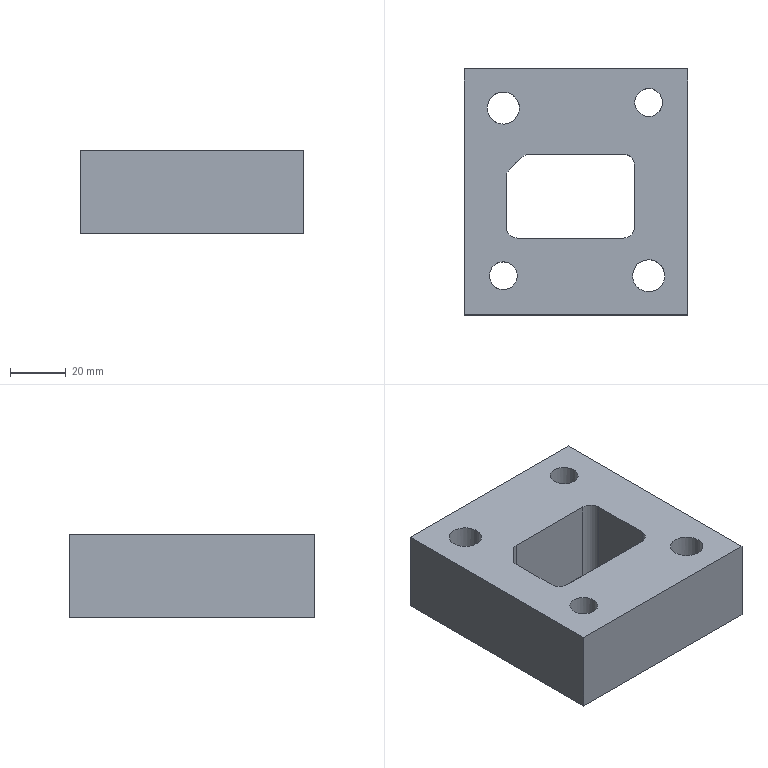Part | NX | features 7 2 | 1 solid | 28 faces | box 80 x 88 x 30 mm | volume 155831 mm3 | plane 15 | cylinder 13 | commonest cylinder face diameters 8 x5 10.001 x2 10.31 x2 11.5 x2 18 x2
STEP:
#1=CARTESIAN_POINT('',(3326.247,115.829,91.));
#2=VERTEX_POINT('',#1);
#3=CARTESIAN_POINT('',(3326.247,110.828,91.));
#4=DIRECTION('',(0.,0.,-1.));
#5=DIRECTION('',(0.,1.,0.));
#6=AXIS2_PLACEMENT_3D('',#3,#4,#5);
#7=CIRCLE('',#6,5.);
#8=EDGE_CURVE('',#2,#2,#7,.T.);
#9=ORIENTED_EDGE('',*,*,#8,.T.);
#10=EDGE_LOOP('',(#9));
#11=FACE_BOUND('',#10,.T.);
#12=CARTESIAN_POINT('',(3274.247,114.578,91.));
#13=VERTEX_POINT('',#12);
#14=CARTESIAN_POINT('',(3274.247,108.828,91.));
#15=DIRECTION('',(0.,0.,1.));
#16=DIRECTION('',(0.,1.,0.));
#17=AXIS2_PLACEMENT_3D('',#14,#15,#16);
#18=CIRCLE('',#17,5.75);
#19=EDGE_CURVE('',#13,#13,#18,.T.);
#20=ORIENTED_EDGE('',*,*,#19,.F.);
#21=EDGE_LOOP('',(#20));
#22=FACE_BOUND('',#21,.T.);
#23=CARTESIAN_POINT('',(3340.247,34.828,91.));
#24=VERTEX_POINT('',#23);
#25=CARTESIAN_POINT('',(3260.247,34.828,91.));
#26=VERTEX_POINT('',#25);
#27=CARTESIAN_POINT('',(3290.247,34.828,91.));
#28=DIRECTION('',(-1.,0.,0.));
#29=VECTOR('',#28,1000.);
#30=LINE('',#27,#29);
#31=EDGE_CURVE('',#24,#26,#30,.T.);
#32=ORIENTED_EDGE('',*,*,#31,.F.);
#33=CARTESIAN_POINT('',(3340.247,122.828,91.));
#34=VERTEX_POINT('',#33);
#35=CARTESIAN_POINT('',(3340.247,77.328,91.));
#36=DIRECTION('',(0.,-1.,0.));
#37=VECTOR('',#36,1000.);
#38=LINE('',#35,#37);
#39=EDGE_CURVE('',#34,#24,#38,.T.);
#40=ORIENTED_EDGE('',*,*,#39,.F.);
#41=CARTESIAN_POINT('',(3260.247,122.828,91.));
#42=VERTEX_POINT('',#41);
#43=CARTESIAN_POINT('',(3290.247,122.828,91.));
#44=DIRECTION('',(1.,0.,0.));
#45=VECTOR('',#44,1000.);
#46=LINE('',#43,#45);
#47=EDGE_CURVE('',#42,#34,#46,.T.);
#48=ORIENTED_EDGE('',*,*,#47,.F.);
#49=CARTESIAN_POINT('',(3260.247,77.328,91.));
#50=DIRECTION('',(0.,1.,0.));
#51=VECTOR('',#50,1000.);
#52=LINE('',#49,#51);
#53=EDGE_CURVE('',#26,#42,#52,.T.);
#54=ORIENTED_EDGE('',*,*,#53,.F.);
#55=EDGE_LOOP('',(#32,#40,#48,#54));
#56=FACE_BOUND('',#55,.T.);
#57=CARTESIAN_POINT('',(3326.247,54.578,91.));
#58=VERTEX_POINT('',#57);
#59=CARTESIAN_POINT('',(3326.247,48.828,91.));
#60=DIRECTION('',(0.,0.,1.));
#61=DIRECTION('',(0.,1.,0.));
#62=AXIS2_PLACEMENT_3D('',#59,#60,#61);
#63=CIRCLE('',#62,5.75);
#64=EDGE_CURVE('',#58,#58,#63,.T.);
#65=ORIENTED_EDGE('',*,*,#64,.F.);
#66=EDGE_LOOP('',(#65));
#67=FACE_BOUND('',#66,.T.);
#68=CARTESIAN_POINT('',(3274.247,53.829,91.));
#69=VERTEX_POINT('',#68);
#70=CARTESIAN_POINT('',(3274.247,48.828,91.));
#71=DIRECTION('',(0.,0.,-1.));
#72=DIRECTION('',(0.,1.,0.));
#73=AXIS2_PLACEMENT_3D('',#70,#71,#72);
#74=CIRCLE('',#73,5.);
#75=EDGE_CURVE('',#69,#69,#74,.T.);
#76=ORIENTED_EDGE('',*,*,#75,.T.);
#77=EDGE_LOOP('',(#76));
#78=FACE_BOUND('',#77,.T.);
#79=CARTESIAN_POINT('',(3317.247,62.328,91.));
#80=VERTEX_POINT('',#79);
#81=CARTESIAN_POINT('',(3321.247,66.328,91.));
#82=VERTEX_POINT('',#81);
#83=CARTESIAN_POINT('',(3317.247,66.328,91.));
#84=DIRECTION('',(0.,0.,1.));
#85=DIRECTION('',(0.,1.,0.));
#86=AXIS2_PLACEMENT_3D('',#83,#84,#85);
#87=CIRCLE('',#86,4.);
#88=EDGE_CURVE('',#80,#82,#87,.T.);
#89=ORIENTED_EDGE('',*,*,#88,.F.);
#90=CARTESIAN_POINT('',(3279.247,62.328,91.));
#91=VERTEX_POINT('',#90);
#92=CARTESIAN_POINT('',(3290.247,62.328,91.));
#93=DIRECTION('',(-1.,0.,0.));
#94=VECTOR('',#93,1000.);
#95=LINE('',#92,#94);
#96=EDGE_CURVE('',#80,#91,#95,.T.);
#97=ORIENTED_EDGE('',*,*,#96,.T.);
#98=CARTESIAN_POINT('',(3275.247,66.328,91.));
#99=VERTEX_POINT('',#98);
#100=CARTESIAN_POINT('',(3279.247,66.328,91.));
#101=DIRECTION('',(0.,0.,1.));
#102=DIRECTION('',(0.,1.,0.));
#103=AXIS2_PLACEMENT_3D('',#100,#101,#102);
#104=CIRCLE('',#103,4.);
#105=EDGE_CURVE('',#99,#91,#104,.T.);
#106=ORIENTED_EDGE('',*,*,#105,.F.);
#107=CARTESIAN_POINT('',(3275.247,84.035,91.));
#108=VERTEX_POINT('',#107);
#109=CARTESIAN_POINT('',(3275.247,77.328,91.));
#110=DIRECTION('',(0.,1.,0.));
#111=VECTOR('',#110,1000.);
#112=LINE('',#109,#111);
#113=EDGE_CURVE('',#99,#108,#112,.T.);
#114=ORIENTED_EDGE('',*,*,#113,.T.);
#115=CARTESIAN_POINT('',(3276.419,86.864,91.));
#116=VERTEX_POINT('',#115);
#117=CARTESIAN_POINT('',(3279.247,84.035,91.));
#118=DIRECTION('',(0.,0.,1.));
#119=DIRECTION('',(0.,1.,0.));
#120=AXIS2_PLACEMENT_3D('',#117,#118,#119);
#121=CIRCLE('',#120,4.);
#122=EDGE_CURVE('',#116,#108,#121,.T.);
#123=ORIENTED_EDGE('',*,*,#122,.F.);
#124=CARTESIAN_POINT('',(3280.711,91.157,91.));
#125=VERTEX_POINT('',#124);
#126=CARTESIAN_POINT('',(3279.815,90.26,91.));
#127=DIRECTION('',(-0.7071,-0.7071,0.));
#128=VECTOR('',#127,1000.);
#129=LINE('',#126,#128);
#130=EDGE_CURVE('',#125,#116,#129,.T.);
#131=ORIENTED_EDGE('',*,*,#130,.F.);
#132=CARTESIAN_POINT('',(3283.54,92.328,91.));
#133=VERTEX_POINT('',#132);
#134=CARTESIAN_POINT('',(3283.54,88.328,91.));
#135=DIRECTION('',(0.,0.,1.));
#136=DIRECTION('',(0.,1.,0.));
#137=AXIS2_PLACEMENT_3D('',#134,#135,#136);
#138=CIRCLE('',#137,4.);
#139=EDGE_CURVE('',#133,#125,#138,.T.);
#140=ORIENTED_EDGE('',*,*,#139,.F.);
#141=CARTESIAN_POINT('',(3317.247,92.328,91.));
#142=VERTEX_POINT('',#141);
#143=CARTESIAN_POINT('',(3290.247,92.328,91.));
#144=DIRECTION('',(1.,0.,0.));
#145=VECTOR('',#144,1000.);
#146=LINE('',#143,#145);
#147=EDGE_CURVE('',#133,#142,#146,.T.);
#148=ORIENTED_EDGE('',*,*,#147,.T.);
#149=CARTESIAN_POINT('',(3321.247,88.328,91.));
#150=VERTEX_POINT('',#149);
#151=CARTESIAN_POINT('',(3317.247,88.328,91.));
#152=DIRECTION('',(0.,0.,1.));
#153=DIRECTION('',(0.,1.,0.));
#154=AXIS2_PLACEMENT_3D('',#151,#152,#153);
#155=CIRCLE('',#154,4.);
#156=EDGE_CURVE('',#150,#142,#155,.T.);
#157=ORIENTED_EDGE('',*,*,#156,.F.);
#158=CARTESIAN_POINT('',(3321.247,77.328,91.));
#159=DIRECTION('',(0.,-1.,0.));
#160=VECTOR('',#159,1000.);
#161=LINE('',#158,#160);
#162=EDGE_CURVE('',#150,#82,#161,.T.);
#163=ORIENTED_EDGE('',*,*,#162,.T.);
#164=EDGE_LOOP('',(#89,#97,#106,#114,#123,#131,#140,#148,#157,#163));
#165=FACE_BOUND('',#164,.T.);
#166=CARTESIAN_POINT('',(3290.247,77.328,91.));
#167=DIRECTION('',(0.,0.,1.));
#168=DIRECTION('',(0.,-1.,0.));
#169=AXIS2_PLACEMENT_3D('',#166,#167,#168);
#170=PLANE('',#169);
#171=ADVANCED_FACE('',(#11,#22,#56,#67,#78,#165),#170,.T.);
#172=CARTESIAN_POINT('',(3331.402,110.828,61.));
#173=VERTEX_POINT('',#172);
#174=CARTESIAN_POINT('',(3326.247,110.828,61.));
#175=DIRECTION('',(0.,0.,1.));
#176=DIRECTION('',(1.,0.,0.));
#177=AXIS2_PLACEMENT_3D('',#174,#175,#176);
#178=CIRCLE('',#177,5.155);
#179=EDGE_CURVE('',#173,#173,#178,.T.);
#180=ORIENTED_EDGE('',*,*,#179,.T.);
#181=EDGE_LOOP('',(#180));
#182=FACE_BOUND('',#181,.T.);
#183=CARTESIAN_POINT('',(3279.402,48.828,61.));
#184=VERTEX_POINT('',#183);
#185=CARTESIAN_POINT('',(3274.247,48.828,61.));
#186=DIRECTION('',(0.,0.,1.));
#187=DIRECTION('',(1.,0.,0.));
#188=AXIS2_PLACEMENT_3D('',#185,#186,#187);
#189=CIRCLE('',#188,5.155);
#190=EDGE_CURVE('',#184,#184,#189,.T.);
#191=ORIENTED_EDGE('',*,*,#190,.T.);
#192=EDGE_LOOP('',(#191));
#193=FACE_BOUND('',#192,.T.);
#194=CARTESIAN_POINT('',(3260.247,122.828,61.));
#195=VERTEX_POINT('',#194);
#196=CARTESIAN_POINT('',(3260.247,34.828,61.));
#197=VERTEX_POINT('',#196);
#198=CARTESIAN_POINT('',(3260.247,-99.672,61.));
#199=DIRECTION('',(0.,-1.,0.));
#200=VECTOR('',#199,1000.);
#201=LINE('',#198,#200);
#202=EDGE_CURVE('',#195,#197,#201,.T.);
#203=ORIENTED_EDGE('',*,*,#202,.F.);
#204=CARTESIAN_POINT('',(3340.247,122.828,61.));
#205=VERTEX_POINT('',#204);
#206=CARTESIAN_POINT('',(3475.247,122.828,61.));
#207=DIRECTION('',(-1.,0.,0.));
#208=VECTOR('',#207,1000.);
#209=LINE('',#206,#208);
#210=EDGE_CURVE('',#205,#195,#209,.T.);
#211=ORIENTED_EDGE('',*,*,#210,.F.);
#212=CARTESIAN_POINT('',(3340.247,34.828,61.));
#213=VERTEX_POINT('',#212);
#214=CARTESIAN_POINT('',(3340.247,-99.672,61.));
#215=DIRECTION('',(0.,1.,0.));
#216=VECTOR('',#215,1000.);
#217=LINE('',#214,#216);
#218=EDGE_CURVE('',#213,#205,#217,.T.);
#219=ORIENTED_EDGE('',*,*,#218,.F.);
#220=CARTESIAN_POINT('',(3475.247,34.828,61.));
#221=DIRECTION('',(1.,0.,0.));
#222=VECTOR('',#221,1000.);
#223=LINE('',#220,#222);
#224=EDGE_CURVE('',#197,#213,#223,.T.);
#225=ORIENTED_EDGE('',*,*,#224,.F.);
#226=EDGE_LOOP('',(#203,#211,#219,#225));
#227=FACE_BOUND('',#226,.T.);
#228=CARTESIAN_POINT('',(3317.247,48.828,61.));
#229=VERTEX_POINT('',#228);
#230=CARTESIAN_POINT('',(3326.247,48.828,61.));
#231=DIRECTION('',(0.,0.,1.));
#232=DIRECTION('',(-1.,0.,0.));
#233=AXIS2_PLACEMENT_3D('',#230,#231,#232);
#234=CIRCLE('',#233,9.);
#235=EDGE_CURVE('',#229,#229,#234,.T.);
#236=ORIENTED_EDGE('',*,*,#235,.T.);
#237=EDGE_LOOP('',(#236));
#238=FACE_BOUND('',#237,.T.);
#239=CARTESIAN_POINT('',(3265.247,108.828,61.));
#240=VERTEX_POINT('',#239);
#241=CARTESIAN_POINT('',(3274.247,108.828,61.));
#242=DIRECTION('',(0.,0.,1.));
#243=DIRECTION('',(-1.,0.,0.));
#244=AXIS2_PLACEMENT_3D('',#241,#242,#243);
#245=CIRCLE('',#244,9.);
#246=EDGE_CURVE('',#240,#240,#245,.T.);
#247=ORIENTED_EDGE('',*,*,#246,.T.);
#248=EDGE_LOOP('',(#247));
#249=FACE_BOUND('',#248,.T.);
#250=CARTESIAN_POINT('',(3321.247,66.328,61.));
#251=VERTEX_POINT('',#250);
#252=CARTESIAN_POINT('',(3317.247,62.328,61.));
#253=VERTEX_POINT('',#252);
#254=CARTESIAN_POINT('',(3317.247,66.328,61.));
#255=DIRECTION('',(0.,0.,-1.));
#256=DIRECTION('',(-1.,0.,0.));
#257=AXIS2_PLACEMENT_3D('',#254,#255,#256);
#258=CIRCLE('',#257,4.);
#259=EDGE_CURVE('',#251,#253,#258,.T.);
#260=ORIENTED_EDGE('',*,*,#259,.F.);
#261=CARTESIAN_POINT('',(3321.247,88.328,61.));
#262=VERTEX_POINT('',#261);
#263=CARTESIAN_POINT('',(3321.247,-99.672,61.));
#264=DIRECTION('',(0.,1.,0.));
#265=VECTOR('',#264,1000.);
#266=LINE('',#263,#265);
#267=EDGE_CURVE('',#251,#262,#266,.T.);
#268=ORIENTED_EDGE('',*,*,#267,.T.);
#269=CARTESIAN_POINT('',(3317.247,92.328,61.));
#270=VERTEX_POINT('',#269);
#271=CARTESIAN_POINT('',(3317.247,88.328,61.));
#272=DIRECTION('',(0.,0.,-1.));
#273=DIRECTION('',(-1.,0.,0.));
#274=AXIS2_PLACEMENT_3D('',#271,#272,#273);
#275=CIRCLE('',#274,4.);
#276=EDGE_CURVE('',#270,#262,#275,.T.);
#277=ORIENTED_EDGE('',*,*,#276,.F.);
#278=CARTESIAN_POINT('',(3283.54,92.328,61.));
#279=VERTEX_POINT('',#278);
#280=CARTESIAN_POINT('',(3475.247,92.328,61.));
#281=DIRECTION('',(-1.,0.,0.));
#282=VECTOR('',#281,1000.);
#283=LINE('',#280,#282);
#284=EDGE_CURVE('',#270,#279,#283,.T.);
#285=ORIENTED_EDGE('',*,*,#284,.T.);
#286=CARTESIAN_POINT('',(3280.711,91.157,61.));
#287=VERTEX_POINT('',#286);
#288=CARTESIAN_POINT('',(3283.54,88.328,61.));
#289=DIRECTION('',(0.,0.,-1.));
#290=DIRECTION('',(-1.,0.,0.));
#291=AXIS2_PLACEMENT_3D('',#288,#289,#290);
#292=CIRCLE('',#291,4.);
#293=EDGE_CURVE('',#287,#279,#292,.T.);
#294=ORIENTED_EDGE('',*,*,#293,.F.);
#295=CARTESIAN_POINT('',(3276.419,86.864,61.));
#296=VERTEX_POINT('',#295);
#297=CARTESIAN_POINT('',(3282.565,93.01,61.));
#298=DIRECTION('',(0.7071,0.7071,0.));
#299=VECTOR('',#298,1000.);
#300=LINE('',#297,#299);
#301=EDGE_CURVE('',#296,#287,#300,.T.);
#302=ORIENTED_EDGE('',*,*,#301,.F.);
#303=CARTESIAN_POINT('',(3275.247,84.035,61.));
#304=VERTEX_POINT('',#303);
#305=CARTESIAN_POINT('',(3279.247,84.035,61.));
#306=DIRECTION('',(0.,0.,-1.));
#307=DIRECTION('',(-1.,0.,0.));
#308=AXIS2_PLACEMENT_3D('',#305,#306,#307);
#309=CIRCLE('',#308,4.);
#310=EDGE_CURVE('',#304,#296,#309,.T.);
#311=ORIENTED_EDGE('',*,*,#310,.F.);
#312=CARTESIAN_POINT('',(3275.247,66.328,61.));
#313=VERTEX_POINT('',#312);
#314=CARTESIAN_POINT('',(3275.247,-99.672,61.));
#315=DIRECTION('',(0.,-1.,0.));
#316=VECTOR('',#315,1000.);
#317=LINE('',#314,#316);
#318=EDGE_CURVE('',#304,#313,#317,.T.);
#319=ORIENTED_EDGE('',*,*,#318,.T.);
#320=CARTESIAN_POINT('',(3279.247,62.328,61.));
#321=VERTEX_POINT('',#320);
#322=CARTESIAN_POINT('',(3279.247,66.328,61.));
#323=DIRECTION('',(0.,0.,-1.));
#324=DIRECTION('',(-1.,0.,0.));
#325=AXIS2_PLACEMENT_3D('',#322,#323,#324);
#326=CIRCLE('',#325,4.);
#327=EDGE_CURVE('',#321,#313,#326,.T.);
#328=ORIENTED_EDGE('',*,*,#327,.F.);
#329=CARTESIAN_POINT('',(3475.247,62.328,61.));
#330=DIRECTION('',(1.,0.,0.));
#331=VECTOR('',#330,1000.);
#332=LINE('',#329,#331);
#333=EDGE_CURVE('',#321,#253,#332,.T.);
#334=ORIENTED_EDGE('',*,*,#333,.T.);
#335=EDGE_LOOP('',(#260,#268,#277,#285,#294,#302,#311,#319,#328,#334));
#336=FACE_BOUND('',#335,.T.);
#337=CARTESIAN_POINT('',(3475.247,-99.672,61.));
#338=DIRECTION('',(0.,0.,-1.));
#339=DIRECTION('',(0.,1.,0.));
#340=AXIS2_PLACEMENT_3D('',#337,#338,#339);
#341=PLANE('',#340);
#342=ADVANCED_FACE('',(#182,#193,#227,#238,#249,#336),#341,.T.);
#343=ORIENTED_EDGE('',*,*,#53,.T.);
#344=CARTESIAN_POINT('',(3260.247,122.828,6.933));
#345=DIRECTION('',(0.,0.,-1.));
#346=VECTOR('',#345,1000.);
#347=LINE('',#344,#346);
#348=EDGE_CURVE('',#42,#195,#347,.T.);
#349=ORIENTED_EDGE('',*,*,#348,.T.);
#350=ORIENTED_EDGE('',*,*,#202,.T.);
#351=CARTESIAN_POINT('',(3260.247,34.828,6.933));
#352=DIRECTION('',(0.,0.,-1.));
#353=VECTOR('',#352,1000.);
#354=LINE('',#351,#353);
#355=EDGE_CURVE('',#26,#197,#354,.T.);
#356=ORIENTED_EDGE('',*,*,#355,.F.);
#357=EDGE_LOOP('',(#343,#349,#350,#356));
#358=FACE_BOUND('',#357,.T.);
#359=CARTESIAN_POINT('',(3260.247,77.328,6.933));
#360=DIRECTION('',(-1.,0.,0.));
#361=DIRECTION('',(0.,0.,-1.));
#362=AXIS2_PLACEMENT_3D('',#359,#360,#361);
#363=PLANE('',#362);
#364=ADVANCED_FACE('',(#358),#363,.T.);
#365=ORIENTED_EDGE('',*,*,#47,.T.);
#366=CARTESIAN_POINT('',(3340.247,122.828,6.933));
#367=DIRECTION('',(0.,0.,-1.));
#368=VECTOR('',#367,1000.);
#369=LINE('',#366,#368);
#370=EDGE_CURVE('',#34,#205,#369,.T.);
#371=ORIENTED_EDGE('',*,*,#370,.T.);
#372=ORIENTED_EDGE('',*,*,#210,.T.);
#373=ORIENTED_EDGE('',*,*,#348,.F.);
#374=EDGE_LOOP('',(#365,#371,#372,#373));
#375=FACE_BOUND('',#374,.T.);
#376=CARTESIAN_POINT('',(3290.247,122.828,6.933));
#377=DIRECTION('',(0.,1.,0.));
#378=DIRECTION('',(0.,0.,1.));
#379=AXIS2_PLACEMENT_3D('',#376,#377,#378);
#380=PLANE('',#379);
#381=ADVANCED_FACE('',(#375),#380,.T.);
#382=ORIENTED_EDGE('',*,*,#39,.T.);
#383=CARTESIAN_POINT('',(3340.247,34.828,6.933));
#384=DIRECTION('',(0.,0.,1.));
#385=VECTOR('',#384,1000.);
#386=LINE('',#383,#385);
#387=EDGE_CURVE('',#213,#24,#386,.T.);
#388=ORIENTED_EDGE('',*,*,#387,.F.);
#389=ORIENTED_EDGE('',*,*,#218,.T.);
#390=ORIENTED_EDGE('',*,*,#370,.F.);
#391=EDGE_LOOP('',(#382,#388,#389,#390));
#392=FACE_BOUND('',#391,.T.);
#393=CARTESIAN_POINT('',(3340.247,77.328,6.933));
#394=DIRECTION('',(1.,0.,0.));
#395=DIRECTION('',(0.,0.,1.));
#396=AXIS2_PLACEMENT_3D('',#393,#394,#395);
#397=PLANE('',#396);
#398=ADVANCED_FACE('',(#392),#397,.T.);
#399=ORIENTED_EDGE('',*,*,#224,.T.);
#400=ORIENTED_EDGE('',*,*,#387,.T.);
#401=ORIENTED_EDGE('',*,*,#31,.T.);
#402=ORIENTED_EDGE('',*,*,#355,.T.);
#403=EDGE_LOOP('',(#399,#400,#401,#402));
#404=FACE_BOUND('',#403,.T.);
#405=CARTESIAN_POINT('',(3290.247,34.828,6.933));
#406=DIRECTION('',(0.,-1.,0.));
#407=DIRECTION('',(0.,0.,-1.));
#408=AXIS2_PLACEMENT_3D('',#405,#406,#407);
#409=PLANE('',#408);
#410=ADVANCED_FACE('',(#404),#409,.T.);
#411=ORIENTED_EDGE('',*,*,#64,.T.);
#412=EDGE_LOOP('',(#411));
#413=FACE_BOUND('',#412,.T.);
#414=CARTESIAN_POINT('',(3331.997,48.828,74.));
#415=VERTEX_POINT('',#414);
#416=CARTESIAN_POINT('',(3326.247,48.828,74.));
#417=DIRECTION('',(0.,0.,1.));
#418=DIRECTION('',(1.,0.,0.));
#419=AXIS2_PLACEMENT_3D('',#416,#417,#418);
#420=CIRCLE('',#419,5.75);
#421=EDGE_CURVE('',#415,#415,#420,.T.);
#422=ORIENTED_EDGE('',*,*,#421,.F.);
#423=EDGE_LOOP('',(#422));
#424=FACE_BOUND('',#423,.T.);
#425=CARTESIAN_POINT('',(3326.247,48.828,51.));
#426=DIRECTION('',(0.,0.,1.));
#427=DIRECTION('',(0.,-1.,0.));
#428=AXIS2_PLACEMENT_3D('',#425,#426,#427);
#429=CYLINDRICAL_SURFACE('',#428,5.75);
#430=ADVANCED_FACE('',(#413,#424),#429,.F.);
#431=ORIENTED_EDGE('',*,*,#421,.T.);
#432=EDGE_LOOP('',(#431));
#433=FACE_BOUND('',#432,.T.);
#434=CARTESIAN_POINT('',(3335.247,48.828,74.));
#435=VERTEX_POINT('',#434);
#436=CARTESIAN_POINT('',(3326.247,48.828,74.));
#437=DIRECTION('',(0.,0.,1.));
#438=DIRECTION('',(1.,0.,0.));
#439=AXIS2_PLACEMENT_3D('',#436,#437,#438);
#440=CIRCLE('',#439,9.);
#441=EDGE_CURVE('',#435,#435,#440,.T.);
#442=ORIENTED_EDGE('',*,*,#441,.F.);
#443=EDGE_LOOP('',(#442));
#444=FACE_BOUND('',#443,.T.);
#445=CARTESIAN_POINT('',(3326.247,48.828,74.));
#446=DIRECTION('',(0.,0.,1.));
#447=DIRECTION('',(0.,-1.,0.));
#448=AXIS2_PLACEMENT_3D('',#445,#446,#447);
#449=PLANE('',#448);
#450=ADVANCED_FACE('',(#433,#444),#449,.F.);
#451=ORIENTED_EDGE('',*,*,#441,.T.);
#452=EDGE_LOOP('',(#451));
#453=FACE_BOUND('',#452,.T.);
#454=ORIENTED_EDGE('',*,*,#235,.F.);
#455=EDGE_LOOP('',(#454));
#456=FACE_BOUND('',#455,.T.);
#457=CARTESIAN_POINT('',(3326.247,48.828,56.));
#458=DIRECTION('',(0.,0.,1.));
#459=DIRECTION('',(0.,-1.,0.));
#460=AXIS2_PLACEMENT_3D('',#457,#458,#459);
#461=CYLINDRICAL_SURFACE('',#460,9.);
#462=ADVANCED_FACE('',(#453,#456),#461,.F.);
#463=CARTESIAN_POINT('',(3279.247,48.828,71.));
#464=VERTEX_POINT('',#463);
#465=CARTESIAN_POINT('',(3274.247,48.828,71.));
#466=DIRECTION('',(0.,0.,-1.));
#467=DIRECTION('',(1.,0.,0.));
#468=AXIS2_PLACEMENT_3D('',#465,#466,#467);
#469=CIRCLE('',#468,5.);
#470=EDGE_CURVE('',#464,#464,#469,.T.);
#471=ORIENTED_EDGE('',*,*,#470,.T.);
#472=EDGE_LOOP('',(#471));
#473=FACE_BOUND('',#472,.T.);
#474=ORIENTED_EDGE('',*,*,#75,.F.);
#475=EDGE_LOOP('',(#474));
#476=FACE_BOUND('',#475,.T.);
#477=CARTESIAN_POINT('',(3274.247,48.828,621.));
#478=DIRECTION('',(0.,0.,-1.));
#479=DIRECTION('',(0.,1.,0.));
#480=AXIS2_PLACEMENT_3D('',#477,#478,#479);
#481=CYLINDRICAL_SURFACE('',#480,5.);
#482=ADVANCED_FACE('',(#473,#476),#481,.F.);
#483=ORIENTED_EDGE('',*,*,#19,.T.);
#484=EDGE_LOOP('',(#483));
#485=FACE_BOUND('',#484,.T.);
#486=CARTESIAN_POINT('',(3279.997,108.828,74.));
#487=VERTEX_POINT('',#486);
#488=CARTESIAN_POINT('',(3274.247,108.828,74.));
#489=DIRECTION('',(0.,0.,1.));
#490=DIRECTION('',(1.,0.,0.));
#491=AXIS2_PLACEMENT_3D('',#488,#489,#490);
#492=CIRCLE('',#491,5.75);
#493=EDGE_CURVE('',#487,#487,#492,.T.);
#494=ORIENTED_EDGE('',*,*,#493,.F.);
#495=EDGE_LOOP('',(#494));
#496=FACE_BOUND('',#495,.T.);
#497=CARTESIAN_POINT('',(3274.247,108.828,51.));
#498=DIRECTION('',(0.,0.,1.));
#499=DIRECTION('',(0.,-1.,0.));
#500=AXIS2_PLACEMENT_3D('',#497,#498,#499);
#501=CYLINDRICAL_SURFACE('',#500,5.75);
#502=ADVANCED_FACE('',(#485,#496),#501,.F.);
#503=ORIENTED_EDGE('',*,*,#493,.T.);
#504=EDGE_LOOP('',(#503));
#505=FACE_BOUND('',#504,.T.);
#506=CARTESIAN_POINT('',(3283.247,108.828,74.));
#507=VERTEX_POINT('',#506);
#508=CARTESIAN_POINT('',(3274.247,108.828,74.));
#509=DIRECTION('',(0.,0.,1.));
#510=DIRECTION('',(1.,0.,0.));
#511=AXIS2_PLACEMENT_3D('',#508,#509,#510);
#512=CIRCLE('',#511,9.);
#513=EDGE_CURVE('',#507,#507,#512,.T.);
#514=ORIENTED_EDGE('',*,*,#513,.F.);
#515=EDGE_LOOP('',(#514));
#516=FACE_BOUND('',#515,.T.);
#517=CARTESIAN_POINT('',(3274.247,108.828,74.));
#518=DIRECTION('',(0.,0.,1.));
#519=DIRECTION('',(0.,-1.,0.));
#520=AXIS2_PLACEMENT_3D('',#517,#518,#519);
#521=PLANE('',#520);
#522=ADVANCED_FACE('',(#505,#516),#521,.F.);
#523=ORIENTED_EDGE('',*,*,#513,.T.);
#524=EDGE_LOOP('',(#523));
#525=FACE_BOUND('',#524,.T.);
#526=ORIENTED_EDGE('',*,*,#246,.F.);
#527=EDGE_LOOP('',(#526));
#528=FACE_BOUND('',#527,.T.);
#529=CARTESIAN_POINT('',(3274.247,108.828,56.));
#530=DIRECTION('',(0.,0.,1.));
#531=DIRECTION('',(0.,-1.,0.));
#532=AXIS2_PLACEMENT_3D('',#529,#530,#531);
#533=CYLINDRICAL_SURFACE('',#532,9.);
#534=ADVANCED_FACE('',(#525,#528),#533,.F.);
#535=CARTESIAN_POINT('',(3331.247,110.828,71.));
#536=VERTEX_POINT('',#535);
#537=CARTESIAN_POINT('',(3326.247,110.828,71.));
#538=DIRECTION('',(0.,0.,-1.));
#539=DIRECTION('',(1.,0.,0.));
#540=AXIS2_PLACEMENT_3D('',#537,#538,#539);
#541=CIRCLE('',#540,5.);
#542=EDGE_CURVE('',#536,#536,#541,.T.);
#543=ORIENTED_EDGE('',*,*,#542,.T.);
#544=EDGE_LOOP('',(#543));
#545=FACE_BOUND('',#544,.T.);
#546=ORIENTED_EDGE('',*,*,#8,.F.);
#547=EDGE_LOOP('',(#546));
#548=FACE_BOUND('',#547,.T.);
#549=CARTESIAN_POINT('',(3326.247,110.828,621.));
#550=DIRECTION('',(0.,0.,-1.));
#551=DIRECTION('',(0.,1.,0.));
#552=AXIS2_PLACEMENT_3D('',#549,#550,#551);
#553=CYLINDRICAL_SURFACE('',#552,5.);
#554=ADVANCED_FACE('',(#545,#548),#553,.F.);
#555=ORIENTED_EDGE('',*,*,#113,.F.);
#556=CARTESIAN_POINT('',(3275.247,66.328,-5.));
#557=DIRECTION('',(0.,0.,-1.));
#558=VECTOR('',#557,1000.);
#559=LINE('',#556,#558);
#560=EDGE_CURVE('',#99,#313,#559,.T.);
#561=ORIENTED_EDGE('',*,*,#560,.T.);
#562=ORIENTED_EDGE('',*,*,#318,.F.);
#563=CARTESIAN_POINT('',(3275.247,84.035,-5.));
#564=DIRECTION('',(0.,0.,1.));
#565=VECTOR('',#564,1000.);
#566=LINE('',#563,#565);
#567=EDGE_CURVE('',#304,#108,#566,.T.);
#568=ORIENTED_EDGE('',*,*,#567,.T.);
#569=EDGE_LOOP('',(#555,#561,#562,#568));
#570=FACE_BOUND('',#569,.T.);
#571=CARTESIAN_POINT('',(3275.247,77.328,-5.));
#572=DIRECTION('',(-1.,0.,0.));
#573=DIRECTION('',(0.,0.,-1.));
#574=AXIS2_PLACEMENT_3D('',#571,#572,#573);
#575=PLANE('',#574);
#576=ADVANCED_FACE('',(#570),#575,.F.);
#577=ORIENTED_EDGE('',*,*,#147,.F.);
#578=CARTESIAN_POINT('',(3283.54,92.328,-5.));
#579=DIRECTION('',(0.,0.,-1.));
#580=VECTOR('',#579,1000.);
#581=LINE('',#578,#580);
#582=EDGE_CURVE('',#133,#279,#581,.T.);
#583=ORIENTED_EDGE('',*,*,#582,.T.);
#584=ORIENTED_EDGE('',*,*,#284,.F.);
#585=CARTESIAN_POINT('',(3317.247,92.328,-5.));
#586=DIRECTION('',(0.,0.,1.));
#587=VECTOR('',#586,1000.);
#588=LINE('',#585,#587);
#589=EDGE_CURVE('',#270,#142,#588,.T.);
#590=ORIENTED_EDGE('',*,*,#589,.T.);
#591=EDGE_LOOP('',(#577,#583,#584,#590));
#592=FACE_BOUND('',#591,.T.);
#593=CARTESIAN_POINT('',(3290.247,92.328,-5.));
#594=DIRECTION('',(0.,1.,0.));
#595=DIRECTION('',(0.,0.,1.));
#596=AXIS2_PLACEMENT_3D('',#593,#594,#595);
#597=PLANE('',#596);
#598=ADVANCED_FACE('',(#592),#597,.F.);
#599=ORIENTED_EDGE('',*,*,#162,.F.);
#600=CARTESIAN_POINT('',(3321.247,88.328,-5.));
#601=DIRECTION('',(0.,0.,-1.));
#602=VECTOR('',#601,1000.);
#603=LINE('',#600,#602);
#604=EDGE_CURVE('',#150,#262,#603,.T.);
#605=ORIENTED_EDGE('',*,*,#604,.T.);
#606=ORIENTED_EDGE('',*,*,#267,.F.);
#607=CARTESIAN_POINT('',(3321.247,66.328,-5.));
#608=DIRECTION('',(0.,0.,1.));
#609=VECTOR('',#608,1000.);
#610=LINE('',#607,#609);
#611=EDGE_CURVE('',#251,#82,#610,.T.);
#612=ORIENTED_EDGE('',*,*,#611,.T.);
#613=EDGE_LOOP('',(#599,#605,#606,#612));
#614=FACE_BOUND('',#613,.T.);
#615=CARTESIAN_POINT('',(3321.247,77.328,-5.));
#616=DIRECTION('',(1.,0.,0.));
#617=DIRECTION('',(0.,0.,1.));
#618=AXIS2_PLACEMENT_3D('',#615,#616,#617);
#619=PLANE('',#618);
#620=ADVANCED_FACE('',(#614),#619,.F.);
#621=ORIENTED_EDGE('',*,*,#333,.F.);
#622=CARTESIAN_POINT('',(3279.247,62.328,-5.));
#623=DIRECTION('',(0.,0.,1.));
#624=VECTOR('',#623,1000.);
#625=LINE('',#622,#624);
#626=EDGE_CURVE('',#321,#91,#625,.T.);
#627=ORIENTED_EDGE('',*,*,#626,.T.);
#628=ORIENTED_EDGE('',*,*,#96,.F.);
#629=CARTESIAN_POINT('',(3317.247,62.328,-5.));
#630=DIRECTION('',(0.,0.,-1.));
#631=VECTOR('',#630,1000.);
#632=LINE('',#629,#631);
#633=EDGE_CURVE('',#80,#253,#632,.T.);
#634=ORIENTED_EDGE('',*,*,#633,.T.);
#635=EDGE_LOOP('',(#621,#627,#628,#634));
#636=FACE_BOUND('',#635,.T.);
#637=CARTESIAN_POINT('',(3290.247,62.328,-5.));
#638=DIRECTION('',(0.,-1.,0.));
#639=DIRECTION('',(0.,0.,-1.));
#640=AXIS2_PLACEMENT_3D('',#637,#638,#639);
#641=PLANE('',#640);
#642=ADVANCED_FACE('',(#636),#641,.F.);
#643=ORIENTED_EDGE('',*,*,#130,.T.);
#644=CARTESIAN_POINT('',(3276.419,86.864,-5.));
#645=DIRECTION('',(0.,0.,-1.));
#646=VECTOR('',#645,1000.);
#647=LINE('',#644,#646);
#648=EDGE_CURVE('',#116,#296,#647,.T.);
#649=ORIENTED_EDGE('',*,*,#648,.T.);
#650=ORIENTED_EDGE('',*,*,#301,.T.);
#651=CARTESIAN_POINT('',(3280.711,91.157,-5.));
#652=DIRECTION('',(0.,0.,1.));
#653=VECTOR('',#652,1000.);
#654=LINE('',#651,#653);
#655=EDGE_CURVE('',#287,#125,#654,.T.);
#656=ORIENTED_EDGE('',*,*,#655,.T.);
#657=EDGE_LOOP('',(#643,#649,#650,#656));
#658=FACE_BOUND('',#657,.T.);
#659=CARTESIAN_POINT('',(3282.565,93.01,-5.));
#660=DIRECTION('',(0.7071,-0.7071,0.));
#661=DIRECTION('',(0.,0.,1.));
#662=AXIS2_PLACEMENT_3D('',#659,#660,#661);
#663=PLANE('',#662);
#664=ADVANCED_FACE('',(#658),#663,.T.);
#665=ORIENTED_EDGE('',*,*,#259,.T.);
#666=ORIENTED_EDGE('',*,*,#633,.F.);
#667=ORIENTED_EDGE('',*,*,#88,.T.);
#668=ORIENTED_EDGE('',*,*,#611,.F.);
#669=EDGE_LOOP('',(#665,#666,#667,#668));
#670=FACE_BOUND('',#669,.T.);
#671=CARTESIAN_POINT('',(3317.247,66.328,-5.));
#672=DIRECTION('',(0.,0.,-1.));
#673=DIRECTION('',(0.,-1.,0.));
#674=AXIS2_PLACEMENT_3D('',#671,#672,#673);
#675=CYLINDRICAL_SURFACE('',#674,4.);
#676=ADVANCED_FACE('',(#670),#675,.F.);
#677=ORIENTED_EDGE('',*,*,#276,.T.);
#678=ORIENTED_EDGE('',*,*,#604,.F.);
#679=ORIENTED_EDGE('',*,*,#156,.T.);
#680=ORIENTED_EDGE('',*,*,#589,.F.);
#681=EDGE_LOOP('',(#677,#678,#679,#680));
#682=FACE_BOUND('',#681,.T.);
#683=CARTESIAN_POINT('',(3317.247,88.328,-5.));
#684=DIRECTION('',(0.,0.,-1.));
#685=DIRECTION('',(0.,-1.,0.));
#686=AXIS2_PLACEMENT_3D('',#683,#684,#685);
#687=CYLINDRICAL_SURFACE('',#686,4.);
#688=ADVANCED_FACE('',(#682),#687,.F.);
#689=ORIENTED_EDGE('',*,*,#293,.T.);
#690=ORIENTED_EDGE('',*,*,#582,.F.);
#691=ORIENTED_EDGE('',*,*,#139,.T.);
#692=ORIENTED_EDGE('',*,*,#655,.F.);
#693=EDGE_LOOP('',(#689,#690,#691,#692));
#694=FACE_BOUND('',#693,.T.);
#695=CARTESIAN_POINT('',(3283.54,88.328,-5.));
#696=DIRECTION('',(0.,0.,1.));
#697=DIRECTION('',(0.,1.,0.));
#698=AXIS2_PLACEMENT_3D('',#695,#696,#697);
#699=CYLINDRICAL_SURFACE('',#698,4.);
#700=ADVANCED_FACE('',(#694),#699,.F.);
#701=ORIENTED_EDGE('',*,*,#122,.T.);
#702=ORIENTED_EDGE('',*,*,#567,.F.);
#703=ORIENTED_EDGE('',*,*,#310,.T.);
#704=ORIENTED_EDGE('',*,*,#648,.F.);
#705=EDGE_LOOP('',(#701,#702,#703,#704));
#706=FACE_BOUND('',#705,.T.);
#707=CARTESIAN_POINT('',(3279.247,84.035,-5.));
#708=DIRECTION('',(0.,0.,-1.));
#709=DIRECTION('',(0.,-1.,0.));
#710=AXIS2_PLACEMENT_3D('',#707,#708,#709);
#711=CYLINDRICAL_SURFACE('',#710,4.);
#712=ADVANCED_FACE('',(#706),#711,.F.);
#713=ORIENTED_EDGE('',*,*,#327,.T.);
#714=ORIENTED_EDGE('',*,*,#560,.F.);
#715=ORIENTED_EDGE('',*,*,#105,.T.);
#716=ORIENTED_EDGE('',*,*,#626,.F.);
#717=EDGE_LOOP('',(#713,#714,#715,#716));
#718=FACE_BOUND('',#717,.T.);
#719=CARTESIAN_POINT('',(3279.247,66.328,-5.));
#720=DIRECTION('',(0.,0.,-1.));
#721=DIRECTION('',(0.,-1.,0.));
#722=AXIS2_PLACEMENT_3D('',#719,#720,#721);
#723=CYLINDRICAL_SURFACE('',#722,4.);
#724=ADVANCED_FACE('',(#718),#723,.F.);
#725=CARTESIAN_POINT('',(3279.402,48.828,71.));
#726=VERTEX_POINT('',#725);
#727=CARTESIAN_POINT('',(3274.247,48.828,71.));
#728=DIRECTION('',(0.,0.,-1.));
#729=DIRECTION('',(1.,0.,0.));
#730=AXIS2_PLACEMENT_3D('',#727,#728,#729);
#731=CIRCLE('',#730,5.155);
#732=EDGE_CURVE('',#726,#726,#731,.T.);
#733=ORIENTED_EDGE('',*,*,#732,.T.);
#734=EDGE_LOOP('',(#733));
#735=FACE_BOUND('',#734,.T.);
#736=ORIENTED_EDGE('',*,*,#470,.F.);
#737=EDGE_LOOP('',(#736));
#738=FACE_BOUND('',#737,.T.);
#739=CARTESIAN_POINT('',(3274.247,48.828,71.));
#740=DIRECTION('',(0.,0.,1.));
#741=DIRECTION('',(-1.,0.,0.));
#742=AXIS2_PLACEMENT_3D('',#739,#740,#741);
#743=PLANE('',#742);
#744=ADVANCED_FACE('',(#735,#738),#743,.F.);
#745=ORIENTED_EDGE('',*,*,#732,.F.);
#746=EDGE_LOOP('',(#745));
#747=FACE_BOUND('',#746,.T.);
#748=ORIENTED_EDGE('',*,*,#190,.F.);
#749=EDGE_LOOP('',(#748));
#750=FACE_BOUND('',#749,.T.);
#751=CARTESIAN_POINT('',(3274.247,48.828,61.));
#752=DIRECTION('',(0.,0.,1.));
#753=DIRECTION('',(-1.,0.,0.));
#754=AXIS2_PLACEMENT_3D('',#751,#752,#753);
#755=CYLINDRICAL_SURFACE('',#754,5.155);
#756=ADVANCED_FACE('',(#747,#750),#755,.F.);
#757=CARTESIAN_POINT('',(3331.402,110.828,71.));
#758=VERTEX_POINT('',#757);
#759=CARTESIAN_POINT('',(3326.247,110.828,71.));
#760=DIRECTION('',(0.,0.,-1.));
#761=DIRECTION('',(1.,0.,0.));
#762=AXIS2_PLACEMENT_3D('',#759,#760,#761);
#763=CIRCLE('',#762,5.155);
#764=EDGE_CURVE('',#758,#758,#763,.T.);
#765=ORIENTED_EDGE('',*,*,#764,.T.);
#766=EDGE_LOOP('',(#765));
#767=FACE_BOUND('',#766,.T.);
#768=ORIENTED_EDGE('',*,*,#542,.F.);
#769=EDGE_LOOP('',(#768));
#770=FACE_BOUND('',#769,.T.);
#771=CARTESIAN_POINT('',(3326.247,110.828,71.));
#772=DIRECTION('',(0.,0.,1.));
#773=DIRECTION('',(-1.,0.,0.));
#774=AXIS2_PLACEMENT_3D('',#771,#772,#773);
#775=PLANE('',#774);
#776=ADVANCED_FACE('',(#767,#770),#775,.F.);
#777=ORIENTED_EDGE('',*,*,#764,.F.);
#778=EDGE_LOOP('',(#777));
#779=FACE_BOUND('',#778,.T.);
#780=ORIENTED_EDGE('',*,*,#179,.F.);
#781=EDGE_LOOP('',(#780));
#782=FACE_BOUND('',#781,.T.);
#783=CARTESIAN_POINT('',(3326.247,110.828,61.));
#784=DIRECTION('',(0.,0.,1.));
#785=DIRECTION('',(-1.,0.,0.));
#786=AXIS2_PLACEMENT_3D('',#783,#784,#785);
#787=CYLINDRICAL_SURFACE('',#786,5.155);
#788=ADVANCED_FACE('',(#779,#782),#787,.F.);
#789=CLOSED_SHELL('',(#171,#342,#364,#381,#398,#410,#430,#450,#462,#482,#502,#522,#534,#554,#576,#598,#620,#642,#664,#676,#688,#700,#712,#724,#744,#756,#776,#788));
#790=MANIFOLD_SOLID_BREP('',#789);
#791=(LENGTH_UNIT()NAMED_UNIT(*)SI_UNIT(.MILLI.,.METRE.));
#792=UNCERTAINTY_MEASURE_WITH_UNIT(LENGTH_MEASURE(0.00001),#791,'','');
#793=(NAMED_UNIT(*)PLANE_ANGLE_UNIT()SI_UNIT($,.RADIAN.));
#794=(NAMED_UNIT(*)SI_UNIT($,.STERADIAN.)SOLID_ANGLE_UNIT());
#795=(GEOMETRIC_REPRESENTATION_CONTEXT(3)GLOBAL_UNCERTAINTY_ASSIGNED_CONTEXT((#792))GLOBAL_UNIT_ASSIGNED_CONTEXT((#791,#793,#794))REPRESENTATION_CONTEXT('',''));
#796=ADVANCED_BREP_SHAPE_REPRESENTATION('',(#790),#795);